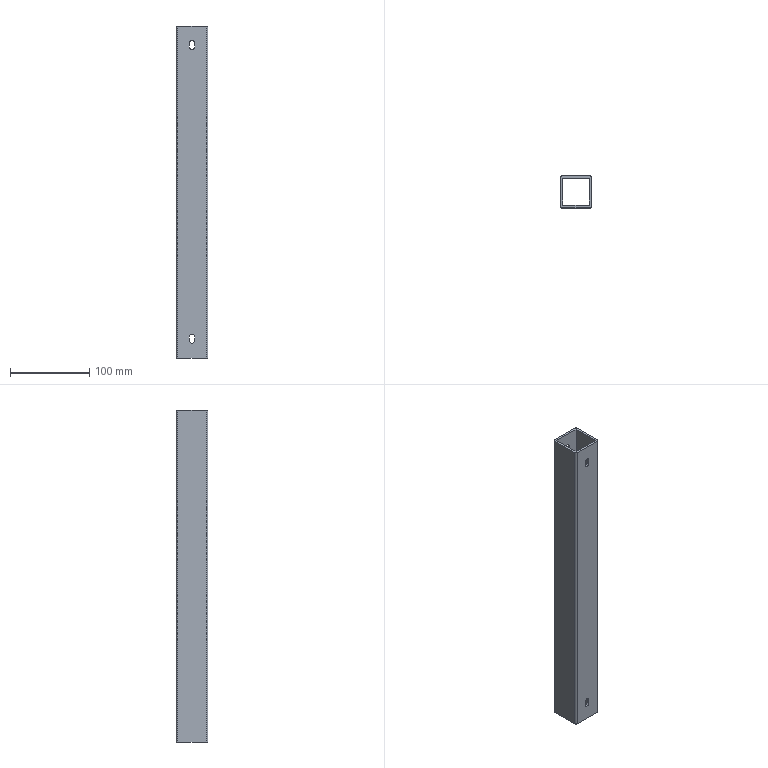Part | STEP file | X77-09102 | 1 solid | 34 faces | box 40 x 40 x 420 mm | volume 183605 mm3 | plane 18 | cylinder 16 | commonest cylinder face diameters 6.5 x6 12 x6 4 x4
STEP:
#1=CARTESIAN_POINT('',(20.,0.,401.386));
#2=VERTEX_POINT('',#1);
#3=CARTESIAN_POINT('',(23.25,0.,398.136));
#4=VERTEX_POINT('',#3);
#5=CARTESIAN_POINT('',(20.,0.,398.136));
#6=DIRECTION('',(0.,1.,0.));
#7=DIRECTION('',(0.,0.,1.));
#8=AXIS2_PLACEMENT_3D('',#5,#6,#7);
#9=CIRCLE('',#8,3.25);
#10=EDGE_CURVE('',#2,#4,#9,.T.);
#11=ORIENTED_EDGE('',*,*,#10,.F.);
#12=CARTESIAN_POINT('',(20.,3.,401.386));
#13=VERTEX_POINT('',#12);
#14=CARTESIAN_POINT('',(20.,-7.,401.386));
#15=DIRECTION('',(0.,1.,0.));
#16=VECTOR('',#15,1000.);
#17=LINE('',#14,#16);
#18=EDGE_CURVE('',#2,#13,#17,.T.);
#19=ORIENTED_EDGE('',*,*,#18,.T.);
#20=CARTESIAN_POINT('',(23.25,3.,398.136));
#21=VERTEX_POINT('',#20);
#22=CARTESIAN_POINT('',(20.,3.,398.136));
#23=DIRECTION('',(0.,1.,0.));
#24=DIRECTION('',(0.,0.,1.));
#25=AXIS2_PLACEMENT_3D('',#22,#23,#24);
#26=CIRCLE('',#25,3.25);
#27=EDGE_CURVE('',#13,#21,#26,.T.);
#28=ORIENTED_EDGE('',*,*,#27,.T.);
#29=CARTESIAN_POINT('',(23.25,-7.,398.136));
#30=DIRECTION('',(0.,1.,0.));
#31=VECTOR('',#30,1000.);
#32=LINE('',#29,#31);
#33=EDGE_CURVE('',#4,#21,#32,.T.);
#34=ORIENTED_EDGE('',*,*,#33,.F.);
#35=EDGE_LOOP('',(#11,#19,#28,#34));
#36=FACE_OUTER_BOUND('',#35,.T.);
#37=CARTESIAN_POINT('',(20.,-7.,398.136));
#38=DIRECTION('',(0.,1.,0.));
#39=DIRECTION('',(0.,0.,1.));
#40=AXIS2_PLACEMENT_3D('',#37,#38,#39);
#41=CYLINDRICAL_SURFACE('',#40,3.25);
#42=ADVANCED_FACE('',(#36),#41,.F.);
#43=CARTESIAN_POINT('',(20.,0.,30.1));
#44=VERTEX_POINT('',#43);
#45=CARTESIAN_POINT('',(23.25,0.,26.85));
#46=VERTEX_POINT('',#45);
#47=CARTESIAN_POINT('',(20.,0.,26.85));
#48=DIRECTION('',(0.,1.,0.));
#49=DIRECTION('',(0.,0.,1.));
#50=AXIS2_PLACEMENT_3D('',#47,#48,#49);
#51=CIRCLE('',#50,3.25);
#52=EDGE_CURVE('',#44,#46,#51,.T.);
#53=ORIENTED_EDGE('',*,*,#52,.F.);
#54=CARTESIAN_POINT('',(20.,3.,30.1));
#55=VERTEX_POINT('',#54);
#56=CARTESIAN_POINT('',(20.,-7.,30.1));
#57=DIRECTION('',(0.,1.,0.));
#58=VECTOR('',#57,1000.);
#59=LINE('',#56,#58);
#60=EDGE_CURVE('',#44,#55,#59,.T.);
#61=ORIENTED_EDGE('',*,*,#60,.T.);
#62=CARTESIAN_POINT('',(23.25,3.,26.85));
#63=VERTEX_POINT('',#62);
#64=CARTESIAN_POINT('',(20.,3.,26.85));
#65=DIRECTION('',(0.,1.,0.));
#66=DIRECTION('',(0.,0.,1.));
#67=AXIS2_PLACEMENT_3D('',#64,#65,#66);
#68=CIRCLE('',#67,3.25);
#69=EDGE_CURVE('',#55,#63,#68,.T.);
#70=ORIENTED_EDGE('',*,*,#69,.T.);
#71=CARTESIAN_POINT('',(23.25,-7.,26.85));
#72=DIRECTION('',(0.,1.,0.));
#73=VECTOR('',#72,1000.);
#74=LINE('',#71,#73);
#75=EDGE_CURVE('',#46,#63,#74,.T.);
#76=ORIENTED_EDGE('',*,*,#75,.F.);
#77=EDGE_LOOP('',(#53,#61,#70,#76));
#78=FACE_OUTER_BOUND('',#77,.T.);
#79=CARTESIAN_POINT('',(20.,-7.,26.85));
#80=DIRECTION('',(0.,1.,0.));
#81=DIRECTION('',(0.,0.,1.));
#82=AXIS2_PLACEMENT_3D('',#79,#80,#81);
#83=CYLINDRICAL_SURFACE('',#82,3.25);
#84=ADVANCED_FACE('',(#78),#83,.F.);
#85=CARTESIAN_POINT('',(26.,37.,398.136));
#86=VERTEX_POINT('',#85);
#87=CARTESIAN_POINT('',(20.,37.,404.136));
#88=VERTEX_POINT('',#87);
#89=CARTESIAN_POINT('',(20.,37.,398.136));
#90=DIRECTION('',(0.,-1.,0.));
#91=DIRECTION('',(0.,0.,-1.));
#92=AXIS2_PLACEMENT_3D('',#89,#90,#91);
#93=CIRCLE('',#92,6.);
#94=EDGE_CURVE('',#86,#88,#93,.T.);
#95=ORIENTED_EDGE('',*,*,#94,.T.);
#96=CARTESIAN_POINT('',(20.,40.,404.136));
#97=VERTEX_POINT('',#96);
#98=CARTESIAN_POINT('',(20.,30.,404.136));
#99=DIRECTION('',(0.,1.,0.));
#100=VECTOR('',#99,1000.);
#101=LINE('',#98,#100);
#102=EDGE_CURVE('',#88,#97,#101,.T.);
#103=ORIENTED_EDGE('',*,*,#102,.T.);
#104=CARTESIAN_POINT('',(26.,40.,398.136));
#105=VERTEX_POINT('',#104);
#106=CARTESIAN_POINT('',(20.,40.,398.136));
#107=DIRECTION('',(0.,1.,0.));
#108=DIRECTION('',(0.,0.,1.));
#109=AXIS2_PLACEMENT_3D('',#106,#107,#108);
#110=CIRCLE('',#109,6.);
#111=EDGE_CURVE('',#97,#105,#110,.T.);
#112=ORIENTED_EDGE('',*,*,#111,.T.);
#113=CARTESIAN_POINT('',(26.,30.,398.136));
#114=DIRECTION('',(0.,1.,0.));
#115=VECTOR('',#114,1000.);
#116=LINE('',#113,#115);
#117=EDGE_CURVE('',#86,#105,#116,.T.);
#118=ORIENTED_EDGE('',*,*,#117,.F.);
#119=EDGE_LOOP('',(#95,#103,#112,#118));
#120=FACE_OUTER_BOUND('',#119,.T.);
#121=CARTESIAN_POINT('',(20.,30.,398.136));
#122=DIRECTION('',(0.,1.,0.));
#123=DIRECTION('',(0.,0.,1.));
#124=AXIS2_PLACEMENT_3D('',#121,#122,#123);
#125=CYLINDRICAL_SURFACE('',#124,6.);
#126=ADVANCED_FACE('',(#120),#125,.F.);
#127=CARTESIAN_POINT('',(26.,37.,26.85));
#128=VERTEX_POINT('',#127);
#129=CARTESIAN_POINT('',(20.,37.,32.85));
#130=VERTEX_POINT('',#129);
#131=CARTESIAN_POINT('',(20.,37.,26.85));
#132=DIRECTION('',(0.,-1.,0.));
#133=DIRECTION('',(0.,0.,-1.));
#134=AXIS2_PLACEMENT_3D('',#131,#132,#133);
#135=CIRCLE('',#134,6.);
#136=EDGE_CURVE('',#128,#130,#135,.T.);
#137=ORIENTED_EDGE('',*,*,#136,.T.);
#138=CARTESIAN_POINT('',(20.,40.,32.85));
#139=VERTEX_POINT('',#138);
#140=CARTESIAN_POINT('',(20.,30.,32.85));
#141=DIRECTION('',(0.,1.,0.));
#142=VECTOR('',#141,1000.);
#143=LINE('',#140,#142);
#144=EDGE_CURVE('',#130,#139,#143,.T.);
#145=ORIENTED_EDGE('',*,*,#144,.T.);
#146=CARTESIAN_POINT('',(26.,40.,26.85));
#147=VERTEX_POINT('',#146);
#148=CARTESIAN_POINT('',(20.,40.,26.85));
#149=DIRECTION('',(0.,1.,0.));
#150=DIRECTION('',(0.,0.,1.));
#151=AXIS2_PLACEMENT_3D('',#148,#149,#150);
#152=CIRCLE('',#151,6.);
#153=EDGE_CURVE('',#139,#147,#152,.T.);
#154=ORIENTED_EDGE('',*,*,#153,.T.);
#155=CARTESIAN_POINT('',(26.,30.,26.85));
#156=DIRECTION('',(0.,1.,0.));
#157=VECTOR('',#156,1000.);
#158=LINE('',#155,#157);
#159=EDGE_CURVE('',#128,#147,#158,.T.);
#160=ORIENTED_EDGE('',*,*,#159,.F.);
#161=EDGE_LOOP('',(#137,#145,#154,#160));
#162=FACE_OUTER_BOUND('',#161,.T.);
#163=CARTESIAN_POINT('',(20.,30.,26.85));
#164=DIRECTION('',(0.,1.,0.));
#165=DIRECTION('',(0.,0.,1.));
#166=AXIS2_PLACEMENT_3D('',#163,#164,#165);
#167=CYLINDRICAL_SURFACE('',#166,6.);
#168=ADVANCED_FACE('',(#162),#167,.F.);
#169=CARTESIAN_POINT('',(0.,2.,420.));
#170=VERTEX_POINT('',#169);
#171=CARTESIAN_POINT('',(2.,0.,420.));
#172=VERTEX_POINT('',#171);
#173=CARTESIAN_POINT('',(2.,2.,420.));
#174=DIRECTION('',(0.,0.,1.));
#175=DIRECTION('',(1.,0.,0.));
#176=AXIS2_PLACEMENT_3D('',#173,#174,#175);
#177=CIRCLE('',#176,2.);
#178=EDGE_CURVE('',#170,#172,#177,.T.);
#179=ORIENTED_EDGE('',*,*,#178,.T.);
#180=CARTESIAN_POINT('',(38.,0.,420.));
#181=VERTEX_POINT('',#180);
#182=CARTESIAN_POINT('',(2.,0.,420.));
#183=DIRECTION('',(1.,0.,0.));
#184=VECTOR('',#183,1000.);
#185=LINE('',#182,#184);
#186=EDGE_CURVE('',#172,#181,#185,.T.);
#187=ORIENTED_EDGE('',*,*,#186,.T.);
#188=CARTESIAN_POINT('',(40.,2.,420.));
#189=VERTEX_POINT('',#188);
#190=CARTESIAN_POINT('',(38.,2.,420.));
#191=DIRECTION('',(0.,0.,1.));
#192=DIRECTION('',(1.,0.,0.));
#193=AXIS2_PLACEMENT_3D('',#190,#191,#192);
#194=CIRCLE('',#193,2.);
#195=EDGE_CURVE('',#181,#189,#194,.T.);
#196=ORIENTED_EDGE('',*,*,#195,.T.);
#197=CARTESIAN_POINT('',(40.,38.,420.));
#198=VERTEX_POINT('',#197);
#199=CARTESIAN_POINT('',(40.,2.,420.));
#200=DIRECTION('',(0.,1.,0.));
#201=VECTOR('',#200,1000.);
#202=LINE('',#199,#201);
#203=EDGE_CURVE('',#189,#198,#202,.T.);
#204=ORIENTED_EDGE('',*,*,#203,.T.);
#205=CARTESIAN_POINT('',(38.,40.,420.));
#206=VERTEX_POINT('',#205);
#207=CARTESIAN_POINT('',(38.,38.,420.));
#208=DIRECTION('',(0.,0.,1.));
#209=DIRECTION('',(1.,0.,0.));
#210=AXIS2_PLACEMENT_3D('',#207,#208,#209);
#211=CIRCLE('',#210,2.);
#212=EDGE_CURVE('',#198,#206,#211,.T.);
#213=ORIENTED_EDGE('',*,*,#212,.T.);
#214=CARTESIAN_POINT('',(2.,40.,420.));
#215=VERTEX_POINT('',#214);
#216=CARTESIAN_POINT('',(2.,40.,420.));
#217=DIRECTION('',(-1.,0.,0.));
#218=VECTOR('',#217,1000.);
#219=LINE('',#216,#218);
#220=EDGE_CURVE('',#206,#215,#219,.T.);
#221=ORIENTED_EDGE('',*,*,#220,.T.);
#222=CARTESIAN_POINT('',(0.,38.,420.));
#223=VERTEX_POINT('',#222);
#224=CARTESIAN_POINT('',(2.,38.,420.));
#225=DIRECTION('',(0.,0.,1.));
#226=DIRECTION('',(-1.,0.,0.));
#227=AXIS2_PLACEMENT_3D('',#224,#225,#226);
#228=CIRCLE('',#227,2.);
#229=EDGE_CURVE('',#215,#223,#228,.T.);
#230=ORIENTED_EDGE('',*,*,#229,.T.);
#231=CARTESIAN_POINT('',(0.,2.,420.));
#232=DIRECTION('',(0.,-1.,0.));
#233=VECTOR('',#232,1000.);
#234=LINE('',#231,#233);
#235=EDGE_CURVE('',#223,#170,#234,.T.);
#236=ORIENTED_EDGE('',*,*,#235,.T.);
#237=EDGE_LOOP('',(#179,#187,#196,#204,#213,#221,#230,#236));
#238=FACE_OUTER_BOUND('',#237,.T.);
#239=CARTESIAN_POINT('',(3.,3.,420.));
#240=VERTEX_POINT('',#239);
#241=CARTESIAN_POINT('',(37.,3.,420.));
#242=VERTEX_POINT('',#241);
#243=CARTESIAN_POINT('',(3.,3.,420.));
#244=DIRECTION('',(1.,0.,0.));
#245=VECTOR('',#244,1000.);
#246=LINE('',#243,#245);
#247=EDGE_CURVE('',#240,#242,#246,.T.);
#248=ORIENTED_EDGE('',*,*,#247,.F.);
#249=CARTESIAN_POINT('',(3.,37.,420.));
#250=VERTEX_POINT('',#249);
#251=CARTESIAN_POINT('',(3.,3.,420.));
#252=DIRECTION('',(0.,-1.,0.));
#253=VECTOR('',#252,1000.);
#254=LINE('',#251,#253);
#255=EDGE_CURVE('',#250,#240,#254,.T.);
#256=ORIENTED_EDGE('',*,*,#255,.F.);
#257=CARTESIAN_POINT('',(37.,37.,420.));
#258=VERTEX_POINT('',#257);
#259=CARTESIAN_POINT('',(3.,37.,420.));
#260=DIRECTION('',(-1.,0.,0.));
#261=VECTOR('',#260,1000.);
#262=LINE('',#259,#261);
#263=EDGE_CURVE('',#258,#250,#262,.T.);
#264=ORIENTED_EDGE('',*,*,#263,.F.);
#265=CARTESIAN_POINT('',(37.,3.,420.));
#266=DIRECTION('',(0.,1.,0.));
#267=VECTOR('',#266,1000.);
#268=LINE('',#265,#267);
#269=EDGE_CURVE('',#242,#258,#268,.T.);
#270=ORIENTED_EDGE('',*,*,#269,.F.);
#271=EDGE_LOOP('',(#248,#256,#264,#270));
#272=FACE_BOUND('',#271,.T.);
#273=CARTESIAN_POINT('',(2.,2.,420.));
#274=DIRECTION('',(0.,0.,1.));
#275=DIRECTION('',(1.,0.,0.));
#276=AXIS2_PLACEMENT_3D('',#273,#274,#275);
#277=PLANE('',#276);
#278=ADVANCED_FACE('',(#238,#272),#277,.T.);
#279=CARTESIAN_POINT('',(0.,2.,0.));
#280=VERTEX_POINT('',#279);
#281=CARTESIAN_POINT('',(2.,0.,0.));
#282=VERTEX_POINT('',#281);
#283=CARTESIAN_POINT('',(2.,2.,0.));
#284=DIRECTION('',(0.,0.,1.));
#285=DIRECTION('',(1.,0.,0.));
#286=AXIS2_PLACEMENT_3D('',#283,#284,#285);
#287=CIRCLE('',#286,2.);
#288=EDGE_CURVE('',#280,#282,#287,.T.);
#289=ORIENTED_EDGE('',*,*,#288,.F.);
#290=CARTESIAN_POINT('',(0.,38.,0.));
#291=VERTEX_POINT('',#290);
#292=CARTESIAN_POINT('',(0.,2.,0.));
#293=DIRECTION('',(0.,-1.,0.));
#294=VECTOR('',#293,1000.);
#295=LINE('',#292,#294);
#296=EDGE_CURVE('',#291,#280,#295,.T.);
#297=ORIENTED_EDGE('',*,*,#296,.F.);
#298=CARTESIAN_POINT('',(2.,40.,0.));
#299=VERTEX_POINT('',#298);
#300=CARTESIAN_POINT('',(2.,38.,0.));
#301=DIRECTION('',(0.,0.,1.));
#302=DIRECTION('',(-1.,0.,0.));
#303=AXIS2_PLACEMENT_3D('',#300,#301,#302);
#304=CIRCLE('',#303,2.);
#305=EDGE_CURVE('',#299,#291,#304,.T.);
#306=ORIENTED_EDGE('',*,*,#305,.F.);
#307=CARTESIAN_POINT('',(38.,40.,0.));
#308=VERTEX_POINT('',#307);
#309=CARTESIAN_POINT('',(2.,40.,0.));
#310=DIRECTION('',(-1.,0.,0.));
#311=VECTOR('',#310,1000.);
#312=LINE('',#309,#311);
#313=EDGE_CURVE('',#308,#299,#312,.T.);
#314=ORIENTED_EDGE('',*,*,#313,.F.);
#315=CARTESIAN_POINT('',(40.,38.,0.));
#316=VERTEX_POINT('',#315);
#317=CARTESIAN_POINT('',(38.,38.,0.));
#318=DIRECTION('',(0.,0.,1.));
#319=DIRECTION('',(1.,0.,0.));
#320=AXIS2_PLACEMENT_3D('',#317,#318,#319);
#321=CIRCLE('',#320,2.);
#322=EDGE_CURVE('',#316,#308,#321,.T.);
#323=ORIENTED_EDGE('',*,*,#322,.F.);
#324=CARTESIAN_POINT('',(40.,2.,0.));
#325=VERTEX_POINT('',#324);
#326=CARTESIAN_POINT('',(40.,2.,0.));
#327=DIRECTION('',(0.,1.,0.));
#328=VECTOR('',#327,1000.);
#329=LINE('',#326,#328);
#330=EDGE_CURVE('',#325,#316,#329,.T.);
#331=ORIENTED_EDGE('',*,*,#330,.F.);
#332=CARTESIAN_POINT('',(38.,0.,0.));
#333=VERTEX_POINT('',#332);
#334=CARTESIAN_POINT('',(38.,2.,0.));
#335=DIRECTION('',(0.,0.,1.));
#336=DIRECTION('',(1.,0.,0.));
#337=AXIS2_PLACEMENT_3D('',#334,#335,#336);
#338=CIRCLE('',#337,2.);
#339=EDGE_CURVE('',#333,#325,#338,.T.);
#340=ORIENTED_EDGE('',*,*,#339,.F.);
#341=CARTESIAN_POINT('',(2.,0.,0.));
#342=DIRECTION('',(1.,0.,0.));
#343=VECTOR('',#342,1000.);
#344=LINE('',#341,#343);
#345=EDGE_CURVE('',#282,#333,#344,.T.);
#346=ORIENTED_EDGE('',*,*,#345,.F.);
#347=EDGE_LOOP('',(#289,#297,#306,#314,#323,#331,#340,#346));
#348=FACE_OUTER_BOUND('',#347,.T.);
#349=CARTESIAN_POINT('',(3.,37.,0.));
#350=VERTEX_POINT('',#349);
#351=CARTESIAN_POINT('',(3.,3.,0.));
#352=VERTEX_POINT('',#351);
#353=CARTESIAN_POINT('',(3.,3.,0.));
#354=DIRECTION('',(0.,-1.,0.));
#355=VECTOR('',#354,1000.);
#356=LINE('',#353,#355);
#357=EDGE_CURVE('',#350,#352,#356,.T.);
#358=ORIENTED_EDGE('',*,*,#357,.T.);
#359=CARTESIAN_POINT('',(37.,3.,0.));
#360=VERTEX_POINT('',#359);
#361=CARTESIAN_POINT('',(3.,3.,0.));
#362=DIRECTION('',(1.,0.,0.));
#363=VECTOR('',#362,1000.);
#364=LINE('',#361,#363);
#365=EDGE_CURVE('',#352,#360,#364,.T.);
#366=ORIENTED_EDGE('',*,*,#365,.T.);
#367=CARTESIAN_POINT('',(37.,37.,0.));
#368=VERTEX_POINT('',#367);
#369=CARTESIAN_POINT('',(37.,3.,0.));
#370=DIRECTION('',(0.,1.,0.));
#371=VECTOR('',#370,1000.);
#372=LINE('',#369,#371);
#373=EDGE_CURVE('',#360,#368,#372,.T.);
#374=ORIENTED_EDGE('',*,*,#373,.T.);
#375=CARTESIAN_POINT('',(3.,37.,0.));
#376=DIRECTION('',(-1.,0.,0.));
#377=VECTOR('',#376,1000.);
#378=LINE('',#375,#377);
#379=EDGE_CURVE('',#368,#350,#378,.T.);
#380=ORIENTED_EDGE('',*,*,#379,.T.);
#381=EDGE_LOOP('',(#358,#366,#374,#380));
#382=FACE_BOUND('',#381,.T.);
#383=CARTESIAN_POINT('',(2.,2.,0.));
#384=DIRECTION('',(0.,0.,1.));
#385=DIRECTION('',(1.,0.,0.));
#386=AXIS2_PLACEMENT_3D('',#383,#384,#385);
#387=PLANE('',#386);
#388=ADVANCED_FACE('',(#348,#382),#387,.F.);
#389=ORIENTED_EDGE('',*,*,#288,.T.);
#390=CARTESIAN_POINT('',(2.,0.,420.));
#391=DIRECTION('',(0.,0.,-1.));
#392=VECTOR('',#391,1000.);
#393=LINE('',#390,#392);
#394=EDGE_CURVE('',#172,#282,#393,.T.);
#395=ORIENTED_EDGE('',*,*,#394,.F.);
#396=ORIENTED_EDGE('',*,*,#178,.F.);
#397=CARTESIAN_POINT('',(0.,2.,420.));
#398=DIRECTION('',(0.,0.,-1.));
#399=VECTOR('',#398,1000.);
#400=LINE('',#397,#399);
#401=EDGE_CURVE('',#170,#280,#400,.T.);
#402=ORIENTED_EDGE('',*,*,#401,.T.);
#403=EDGE_LOOP('',(#389,#395,#396,#402));
#404=FACE_OUTER_BOUND('',#403,.T.);
#405=CARTESIAN_POINT('',(2.,2.,420.));
#406=DIRECTION('',(0.,0.,-1.));
#407=DIRECTION('',(-1.,0.,0.));
#408=AXIS2_PLACEMENT_3D('',#405,#406,#407);
#409=CYLINDRICAL_SURFACE('',#408,2.);
#410=ADVANCED_FACE('',(#404),#409,.T.);
#411=CARTESIAN_POINT('',(16.75,0.,393.136));
#412=VERTEX_POINT('',#411);
#413=CARTESIAN_POINT('',(16.75,0.,398.136));
#414=VERTEX_POINT('',#413);
#415=CARTESIAN_POINT('',(16.75,0.,420.));
#416=DIRECTION('',(0.,0.,1.));
#417=VECTOR('',#416,1000.);
#418=LINE('',#415,#417);
#419=EDGE_CURVE('',#412,#414,#418,.T.);
#420=ORIENTED_EDGE('',*,*,#419,.T.);
#421=CARTESIAN_POINT('',(20.,0.,398.136));
#422=DIRECTION('',(0.,1.,0.));
#423=DIRECTION('',(0.,0.,1.));
#424=AXIS2_PLACEMENT_3D('',#421,#422,#423);
#425=CIRCLE('',#424,3.25);
#426=EDGE_CURVE('',#414,#2,#425,.T.);
#427=ORIENTED_EDGE('',*,*,#426,.T.);
#428=ORIENTED_EDGE('',*,*,#10,.T.);
#429=CARTESIAN_POINT('',(23.25,0.,393.136));
#430=VERTEX_POINT('',#429);
#431=CARTESIAN_POINT('',(23.25,0.,420.));
#432=DIRECTION('',(0.,0.,-1.));
#433=VECTOR('',#432,1000.);
#434=LINE('',#431,#433);
#435=EDGE_CURVE('',#4,#430,#434,.T.);
#436=ORIENTED_EDGE('',*,*,#435,.T.);
#437=CARTESIAN_POINT('',(20.,0.,393.136));
#438=DIRECTION('',(0.,1.,0.));
#439=DIRECTION('',(0.,0.,1.));
#440=AXIS2_PLACEMENT_3D('',#437,#438,#439);
#441=CIRCLE('',#440,3.25);
#442=EDGE_CURVE('',#430,#412,#441,.T.);
#443=ORIENTED_EDGE('',*,*,#442,.T.);
#444=EDGE_LOOP('',(#420,#427,#428,#436,#443));
#445=FACE_BOUND('',#444,.T.);
#446=CARTESIAN_POINT('',(23.25,0.,21.85));
#447=VERTEX_POINT('',#446);
#448=CARTESIAN_POINT('',(23.25,0.,420.));
#449=DIRECTION('',(0.,0.,-1.));
#450=VECTOR('',#449,1000.);
#451=LINE('',#448,#450);
#452=EDGE_CURVE('',#46,#447,#451,.T.);
#453=ORIENTED_EDGE('',*,*,#452,.T.);
#454=CARTESIAN_POINT('',(16.75,0.,21.85));
#455=VERTEX_POINT('',#454);
#456=CARTESIAN_POINT('',(20.,0.,21.85));
#457=DIRECTION('',(0.,1.,0.));
#458=DIRECTION('',(0.,0.,1.));
#459=AXIS2_PLACEMENT_3D('',#456,#457,#458);
#460=CIRCLE('',#459,3.25);
#461=EDGE_CURVE('',#447,#455,#460,.T.);
#462=ORIENTED_EDGE('',*,*,#461,.T.);
#463=CARTESIAN_POINT('',(16.75,0.,26.85));
#464=VERTEX_POINT('',#463);
#465=CARTESIAN_POINT('',(16.75,0.,420.));
#466=DIRECTION('',(0.,0.,1.));
#467=VECTOR('',#466,1000.);
#468=LINE('',#465,#467);
#469=EDGE_CURVE('',#455,#464,#468,.T.);
#470=ORIENTED_EDGE('',*,*,#469,.T.);
#471=CARTESIAN_POINT('',(20.,0.,26.85));
#472=DIRECTION('',(0.,1.,0.));
#473=DIRECTION('',(0.,0.,1.));
#474=AXIS2_PLACEMENT_3D('',#471,#472,#473);
#475=CIRCLE('',#474,3.25);
#476=EDGE_CURVE('',#464,#44,#475,.T.);
#477=ORIENTED_EDGE('',*,*,#476,.T.);
#478=ORIENTED_EDGE('',*,*,#52,.T.);
#479=EDGE_LOOP('',(#453,#462,#470,#477,#478));
#480=FACE_BOUND('',#479,.T.);
#481=ORIENTED_EDGE('',*,*,#345,.T.);
#482=CARTESIAN_POINT('',(38.,0.,420.));
#483=DIRECTION('',(0.,0.,-1.));
#484=VECTOR('',#483,1000.);
#485=LINE('',#482,#484);
#486=EDGE_CURVE('',#181,#333,#485,.T.);
#487=ORIENTED_EDGE('',*,*,#486,.F.);
#488=ORIENTED_EDGE('',*,*,#186,.F.);
#489=ORIENTED_EDGE('',*,*,#394,.T.);
#490=EDGE_LOOP('',(#481,#487,#488,#489));
#491=FACE_OUTER_BOUND('',#490,.T.);
#492=CARTESIAN_POINT('',(2.,0.,420.));
#493=DIRECTION('',(0.,1.,0.));
#494=DIRECTION('',(0.,0.,1.));
#495=AXIS2_PLACEMENT_3D('',#492,#493,#494);
#496=PLANE('',#495);
#497=ADVANCED_FACE('',(#445,#480,#491),#496,.F.);
#498=ORIENTED_EDGE('',*,*,#339,.T.);
#499=CARTESIAN_POINT('',(40.,2.,420.));
#500=DIRECTION('',(0.,0.,-1.));
#501=VECTOR('',#500,1000.);
#502=LINE('',#499,#501);
#503=EDGE_CURVE('',#189,#325,#502,.T.);
#504=ORIENTED_EDGE('',*,*,#503,.F.);
#505=ORIENTED_EDGE('',*,*,#195,.F.);
#506=ORIENTED_EDGE('',*,*,#486,.T.);
#507=EDGE_LOOP('',(#498,#504,#505,#506));
#508=FACE_OUTER_BOUND('',#507,.T.);
#509=CARTESIAN_POINT('',(38.,2.,420.));
#510=DIRECTION('',(0.,0.,-1.));
#511=DIRECTION('',(-1.,0.,0.));
#512=AXIS2_PLACEMENT_3D('',#509,#510,#511);
#513=CYLINDRICAL_SURFACE('',#512,2.);
#514=ADVANCED_FACE('',(#508),#513,.T.);
#515=ORIENTED_EDGE('',*,*,#330,.T.);
#516=CARTESIAN_POINT('',(40.,38.,420.));
#517=DIRECTION('',(0.,0.,-1.));
#518=VECTOR('',#517,1000.);
#519=LINE('',#516,#518);
#520=EDGE_CURVE('',#198,#316,#519,.T.);
#521=ORIENTED_EDGE('',*,*,#520,.F.);
#522=ORIENTED_EDGE('',*,*,#203,.F.);
#523=ORIENTED_EDGE('',*,*,#503,.T.);
#524=EDGE_LOOP('',(#515,#521,#522,#523));
#525=FACE_OUTER_BOUND('',#524,.T.);
#526=CARTESIAN_POINT('',(40.,2.,420.));
#527=DIRECTION('',(-1.,0.,0.));
#528=DIRECTION('',(0.,-1.,0.));
#529=AXIS2_PLACEMENT_3D('',#526,#527,#528);
#530=PLANE('',#529);
#531=ADVANCED_FACE('',(#525),#530,.F.);
#532=ORIENTED_EDGE('',*,*,#322,.T.);
#533=CARTESIAN_POINT('',(38.,40.,420.));
#534=DIRECTION('',(0.,0.,-1.));
#535=VECTOR('',#534,1000.);
#536=LINE('',#533,#535);
#537=EDGE_CURVE('',#206,#308,#536,.T.);
#538=ORIENTED_EDGE('',*,*,#537,.F.);
#539=ORIENTED_EDGE('',*,*,#212,.F.);
#540=ORIENTED_EDGE('',*,*,#520,.T.);
#541=EDGE_LOOP('',(#532,#538,#539,#540));
#542=FACE_OUTER_BOUND('',#541,.T.);
#543=CARTESIAN_POINT('',(38.,38.,420.));
#544=DIRECTION('',(0.,0.,-1.));
#545=DIRECTION('',(-1.,0.,0.));
#546=AXIS2_PLACEMENT_3D('',#543,#544,#545);
#547=CYLINDRICAL_SURFACE('',#546,2.);
#548=ADVANCED_FACE('',(#542),#547,.T.);
#549=CARTESIAN_POINT('',(14.,40.,393.136));
#550=VERTEX_POINT('',#549);
#551=CARTESIAN_POINT('',(14.,40.,398.136));
#552=VERTEX_POINT('',#551);
#553=CARTESIAN_POINT('',(14.,40.,393.136));
#554=DIRECTION('',(0.,0.,1.));
#555=VECTOR('',#554,1000.);
#556=LINE('',#553,#555);
#557=EDGE_CURVE('',#550,#552,#556,.T.);
#558=ORIENTED_EDGE('',*,*,#557,.F.);
#559=CARTESIAN_POINT('',(26.,40.,393.136));
#560=VERTEX_POINT('',#559);
#561=CARTESIAN_POINT('',(20.,40.,393.136));
#562=DIRECTION('',(0.,1.,0.));
#563=DIRECTION('',(0.,0.,1.));
#564=AXIS2_PLACEMENT_3D('',#561,#562,#563);
#565=CIRCLE('',#564,6.);
#566=EDGE_CURVE('',#560,#550,#565,.T.);
#567=ORIENTED_EDGE('',*,*,#566,.F.);
#568=CARTESIAN_POINT('',(26.,40.,393.136));
#569=DIRECTION('',(0.,0.,-1.));
#570=VECTOR('',#569,1000.);
#571=LINE('',#568,#570);
#572=EDGE_CURVE('',#105,#560,#571,.T.);
#573=ORIENTED_EDGE('',*,*,#572,.F.);
#574=ORIENTED_EDGE('',*,*,#111,.F.);
#575=CARTESIAN_POINT('',(20.,40.,398.136));
#576=DIRECTION('',(0.,1.,0.));
#577=DIRECTION('',(0.,0.,1.));
#578=AXIS2_PLACEMENT_3D('',#575,#576,#577);
#579=CIRCLE('',#578,6.);
#580=EDGE_CURVE('',#552,#97,#579,.T.);
#581=ORIENTED_EDGE('',*,*,#580,.F.);
#582=EDGE_LOOP('',(#558,#567,#573,#574,#581));
#583=FACE_BOUND('',#582,.T.);
#584=CARTESIAN_POINT('',(14.,40.,21.85));
#585=VERTEX_POINT('',#584);
#586=CARTESIAN_POINT('',(14.,40.,26.85));
#587=VERTEX_POINT('',#586);
#588=CARTESIAN_POINT('',(14.,40.,21.85));
#589=DIRECTION('',(0.,0.,1.));
#590=VECTOR('',#589,1000.);
#591=LINE('',#588,#590);
#592=EDGE_CURVE('',#585,#587,#591,.T.);
#593=ORIENTED_EDGE('',*,*,#592,.F.);
#594=CARTESIAN_POINT('',(26.,40.,21.85));
#595=VERTEX_POINT('',#594);
#596=CARTESIAN_POINT('',(20.,40.,21.85));
#597=DIRECTION('',(0.,1.,0.));
#598=DIRECTION('',(0.,0.,1.));
#599=AXIS2_PLACEMENT_3D('',#596,#597,#598);
#600=CIRCLE('',#599,6.);
#601=EDGE_CURVE('',#595,#585,#600,.T.);
#602=ORIENTED_EDGE('',*,*,#601,.F.);
#603=CARTESIAN_POINT('',(26.,40.,21.85));
#604=DIRECTION('',(0.,0.,-1.));
#605=VECTOR('',#604,1000.);
#606=LINE('',#603,#605);
#607=EDGE_CURVE('',#147,#595,#606,.T.);
#608=ORIENTED_EDGE('',*,*,#607,.F.);
#609=ORIENTED_EDGE('',*,*,#153,.F.);
#610=CARTESIAN_POINT('',(20.,40.,26.85));
#611=DIRECTION('',(0.,1.,0.));
#612=DIRECTION('',(0.,0.,1.));
#613=AXIS2_PLACEMENT_3D('',#610,#611,#612);
#614=CIRCLE('',#613,6.);
#615=EDGE_CURVE('',#587,#139,#614,.T.);
#616=ORIENTED_EDGE('',*,*,#615,.F.);
#617=EDGE_LOOP('',(#593,#602,#608,#609,#616));
#618=FACE_BOUND('',#617,.T.);
#619=ORIENTED_EDGE('',*,*,#313,.T.);
#620=CARTESIAN_POINT('',(2.,40.,420.));
#621=DIRECTION('',(0.,0.,-1.));
#622=VECTOR('',#621,1000.);
#623=LINE('',#620,#622);
#624=EDGE_CURVE('',#215,#299,#623,.T.);
#625=ORIENTED_EDGE('',*,*,#624,.F.);
#626=ORIENTED_EDGE('',*,*,#220,.F.);
#627=ORIENTED_EDGE('',*,*,#537,.T.);
#628=EDGE_LOOP('',(#619,#625,#626,#627));
#629=FACE_OUTER_BOUND('',#628,.T.);
#630=CARTESIAN_POINT('',(2.,40.,420.));
#631=DIRECTION('',(0.,-1.,0.));
#632=DIRECTION('',(0.,0.,-1.));
#633=AXIS2_PLACEMENT_3D('',#630,#631,#632);
#634=PLANE('',#633);
#635=ADVANCED_FACE('',(#583,#618,#629),#634,.F.);
#636=ORIENTED_EDGE('',*,*,#305,.T.);
#637=CARTESIAN_POINT('',(0.,38.,420.));
#638=DIRECTION('',(0.,0.,-1.));
#639=VECTOR('',#638,1000.);
#640=LINE('',#637,#639);
#641=EDGE_CURVE('',#223,#291,#640,.T.);
#642=ORIENTED_EDGE('',*,*,#641,.F.);
#643=ORIENTED_EDGE('',*,*,#229,.F.);
#644=ORIENTED_EDGE('',*,*,#624,.T.);
#645=EDGE_LOOP('',(#636,#642,#643,#644));
#646=FACE_OUTER_BOUND('',#645,.T.);
#647=CARTESIAN_POINT('',(2.,38.,420.));
#648=DIRECTION('',(0.,0.,-1.));
#649=DIRECTION('',(-1.,0.,0.));
#650=AXIS2_PLACEMENT_3D('',#647,#648,#649);
#651=CYLINDRICAL_SURFACE('',#650,2.);
#652=ADVANCED_FACE('',(#646),#651,.T.);
#653=ORIENTED_EDGE('',*,*,#296,.T.);
#654=ORIENTED_EDGE('',*,*,#401,.F.);
#655=ORIENTED_EDGE('',*,*,#235,.F.);
#656=ORIENTED_EDGE('',*,*,#641,.T.);
#657=EDGE_LOOP('',(#653,#654,#655,#656));
#658=FACE_OUTER_BOUND('',#657,.T.);
#659=CARTESIAN_POINT('',(0.,2.,420.));
#660=DIRECTION('',(1.,0.,0.));
#661=DIRECTION('',(0.,1.,0.));
#662=AXIS2_PLACEMENT_3D('',#659,#660,#661);
#663=PLANE('',#662);
#664=ADVANCED_FACE('',(#658),#663,.F.);
#665=ORIENTED_EDGE('',*,*,#357,.F.);
#666=CARTESIAN_POINT('',(3.,37.,420.));
#667=DIRECTION('',(0.,0.,-1.));
#668=VECTOR('',#667,1000.);
#669=LINE('',#666,#668);
#670=EDGE_CURVE('',#250,#350,#669,.T.);
#671=ORIENTED_EDGE('',*,*,#670,.F.);
#672=ORIENTED_EDGE('',*,*,#255,.T.);
#673=CARTESIAN_POINT('',(3.,3.,420.));
#674=DIRECTION('',(0.,0.,-1.));
#675=VECTOR('',#674,1000.);
#676=LINE('',#673,#675);
#677=EDGE_CURVE('',#240,#352,#676,.T.);
#678=ORIENTED_EDGE('',*,*,#677,.T.);
#679=EDGE_LOOP('',(#665,#671,#672,#678));
#680=FACE_OUTER_BOUND('',#679,.T.);
#681=CARTESIAN_POINT('',(3.,3.,420.));
#682=DIRECTION('',(1.,0.,0.));
#683=DIRECTION('',(0.,0.,-1.));
#684=AXIS2_PLACEMENT_3D('',#681,#682,#683);
#685=PLANE('',#684);
#686=ADVANCED_FACE('',(#680),#685,.T.);
#687=CARTESIAN_POINT('',(16.75,3.,398.136));
#688=VERTEX_POINT('',#687);
#689=CARTESIAN_POINT('',(20.,3.,398.136));
#690=DIRECTION('',(0.,1.,0.));
#691=DIRECTION('',(0.,0.,1.));
#692=AXIS2_PLACEMENT_3D('',#689,#690,#691);
#693=CIRCLE('',#692,3.25);
#694=EDGE_CURVE('',#688,#13,#693,.T.);
#695=ORIENTED_EDGE('',*,*,#694,.F.);
#696=CARTESIAN_POINT('',(16.75,3.,393.136));
#697=VERTEX_POINT('',#696);
#698=CARTESIAN_POINT('',(16.75,3.,398.136));
#699=DIRECTION('',(0.,0.,1.));
#700=VECTOR('',#699,1000.);
#701=LINE('',#698,#700);
#702=EDGE_CURVE('',#697,#688,#701,.T.);
#703=ORIENTED_EDGE('',*,*,#702,.F.);
#704=CARTESIAN_POINT('',(23.25,3.,393.136));
#705=VERTEX_POINT('',#704);
#706=CARTESIAN_POINT('',(20.,3.,393.136));
#707=DIRECTION('',(0.,1.,0.));
#708=DIRECTION('',(0.,0.,1.));
#709=AXIS2_PLACEMENT_3D('',#706,#707,#708);
#710=CIRCLE('',#709,3.25);
#711=EDGE_CURVE('',#705,#697,#710,.T.);
#712=ORIENTED_EDGE('',*,*,#711,.F.);
#713=CARTESIAN_POINT('',(23.25,3.,398.136));
#714=DIRECTION('',(0.,0.,-1.));
#715=VECTOR('',#714,1000.);
#716=LINE('',#713,#715);
#717=EDGE_CURVE('',#21,#705,#716,.T.);
#718=ORIENTED_EDGE('',*,*,#717,.F.);
#719=ORIENTED_EDGE('',*,*,#27,.F.);
#720=EDGE_LOOP('',(#695,#703,#712,#718,#719));
#721=FACE_BOUND('',#720,.T.);
#722=CARTESIAN_POINT('',(23.25,3.,21.85));
#723=VERTEX_POINT('',#722);
#724=CARTESIAN_POINT('',(16.75,3.,21.85));
#725=VERTEX_POINT('',#724);
#726=CARTESIAN_POINT('',(20.,3.,21.85));
#727=DIRECTION('',(0.,1.,0.));
#728=DIRECTION('',(0.,0.,1.));
#729=AXIS2_PLACEMENT_3D('',#726,#727,#728);
#730=CIRCLE('',#729,3.25);
#731=EDGE_CURVE('',#723,#725,#730,.T.);
#732=ORIENTED_EDGE('',*,*,#731,.F.);
#733=CARTESIAN_POINT('',(23.25,3.,21.85));
#734=DIRECTION('',(0.,0.,-1.));
#735=VECTOR('',#734,1000.);
#736=LINE('',#733,#735);
#737=EDGE_CURVE('',#63,#723,#736,.T.);
#738=ORIENTED_EDGE('',*,*,#737,.F.);
#739=ORIENTED_EDGE('',*,*,#69,.F.);
#740=CARTESIAN_POINT('',(16.75,3.,26.85));
#741=VERTEX_POINT('',#740);
#742=CARTESIAN_POINT('',(20.,3.,26.85));
#743=DIRECTION('',(0.,1.,0.));
#744=DIRECTION('',(0.,0.,1.));
#745=AXIS2_PLACEMENT_3D('',#742,#743,#744);
#746=CIRCLE('',#745,3.25);
#747=EDGE_CURVE('',#741,#55,#746,.T.);
#748=ORIENTED_EDGE('',*,*,#747,.F.);
#749=CARTESIAN_POINT('',(16.75,3.,21.85));
#750=DIRECTION('',(0.,0.,1.));
#751=VECTOR('',#750,1000.);
#752=LINE('',#749,#751);
#753=EDGE_CURVE('',#725,#741,#752,.T.);
#754=ORIENTED_EDGE('',*,*,#753,.F.);
#755=EDGE_LOOP('',(#732,#738,#739,#748,#754));
#756=FACE_BOUND('',#755,.T.);
#757=ORIENTED_EDGE('',*,*,#365,.F.);
#758=ORIENTED_EDGE('',*,*,#677,.F.);
#759=ORIENTED_EDGE('',*,*,#247,.T.);
#760=CARTESIAN_POINT('',(37.,3.,420.));
#761=DIRECTION('',(0.,0.,-1.));
#762=VECTOR('',#761,1000.);
#763=LINE('',#760,#762);
#764=EDGE_CURVE('',#242,#360,#763,.T.);
#765=ORIENTED_EDGE('',*,*,#764,.T.);
#766=EDGE_LOOP('',(#757,#758,#759,#765));
#767=FACE_OUTER_BOUND('',#766,.T.);
#768=CARTESIAN_POINT('',(3.,3.,420.));
#769=DIRECTION('',(0.,1.,0.));
#770=DIRECTION('',(0.,0.,1.));
#771=AXIS2_PLACEMENT_3D('',#768,#769,#770);
#772=PLANE('',#771);
#773=ADVANCED_FACE('',(#721,#756,#767),#772,.T.);
#774=ORIENTED_EDGE('',*,*,#373,.F.);
#775=ORIENTED_EDGE('',*,*,#764,.F.);
#776=ORIENTED_EDGE('',*,*,#269,.T.);
#777=CARTESIAN_POINT('',(37.,37.,420.));
#778=DIRECTION('',(0.,0.,-1.));
#779=VECTOR('',#778,1000.);
#780=LINE('',#777,#779);
#781=EDGE_CURVE('',#258,#368,#780,.T.);
#782=ORIENTED_EDGE('',*,*,#781,.T.);
#783=EDGE_LOOP('',(#774,#775,#776,#782));
#784=FACE_OUTER_BOUND('',#783,.T.);
#785=CARTESIAN_POINT('',(37.,3.,420.));
#786=DIRECTION('',(-1.,0.,0.));
#787=DIRECTION('',(0.,0.,1.));
#788=AXIS2_PLACEMENT_3D('',#785,#786,#787);
#789=PLANE('',#788);
#790=ADVANCED_FACE('',(#784),#789,.T.);
#791=CARTESIAN_POINT('',(14.,37.,393.136));
#792=VERTEX_POINT('',#791);
#793=CARTESIAN_POINT('',(26.,37.,393.136));
#794=VERTEX_POINT('',#793);
#795=CARTESIAN_POINT('',(20.,37.,393.136));
#796=DIRECTION('',(0.,-1.,0.));
#797=DIRECTION('',(0.,0.,-1.));
#798=AXIS2_PLACEMENT_3D('',#795,#796,#797);
#799=CIRCLE('',#798,6.);
#800=EDGE_CURVE('',#792,#794,#799,.T.);
#801=ORIENTED_EDGE('',*,*,#800,.F.);
#802=CARTESIAN_POINT('',(14.,37.,398.136));
#803=VERTEX_POINT('',#802);
#804=CARTESIAN_POINT('',(14.,37.,420.));
#805=DIRECTION('',(0.,0.,-1.));
#806=VECTOR('',#805,1000.);
#807=LINE('',#804,#806);
#808=EDGE_CURVE('',#803,#792,#807,.T.);
#809=ORIENTED_EDGE('',*,*,#808,.F.);
#810=CARTESIAN_POINT('',(20.,37.,398.136));
#811=DIRECTION('',(0.,-1.,0.));
#812=DIRECTION('',(0.,0.,-1.));
#813=AXIS2_PLACEMENT_3D('',#810,#811,#812);
#814=CIRCLE('',#813,6.);
#815=EDGE_CURVE('',#88,#803,#814,.T.);
#816=ORIENTED_EDGE('',*,*,#815,.F.);
#817=ORIENTED_EDGE('',*,*,#94,.F.);
#818=CARTESIAN_POINT('',(26.,37.,420.));
#819=DIRECTION('',(0.,0.,1.));
#820=VECTOR('',#819,1000.);
#821=LINE('',#818,#820);
#822=EDGE_CURVE('',#794,#86,#821,.T.);
#823=ORIENTED_EDGE('',*,*,#822,.F.);
#824=EDGE_LOOP('',(#801,#809,#816,#817,#823));
#825=FACE_BOUND('',#824,.T.);
#826=CARTESIAN_POINT('',(14.,37.,21.85));
#827=VERTEX_POINT('',#826);
#828=CARTESIAN_POINT('',(26.,37.,21.85));
#829=VERTEX_POINT('',#828);
#830=CARTESIAN_POINT('',(20.,37.,21.85));
#831=DIRECTION('',(0.,-1.,0.));
#832=DIRECTION('',(0.,0.,-1.));
#833=AXIS2_PLACEMENT_3D('',#830,#831,#832);
#834=CIRCLE('',#833,6.);
#835=EDGE_CURVE('',#827,#829,#834,.T.);
#836=ORIENTED_EDGE('',*,*,#835,.F.);
#837=CARTESIAN_POINT('',(14.,37.,26.85));
#838=VERTEX_POINT('',#837);
#839=CARTESIAN_POINT('',(14.,37.,420.));
#840=DIRECTION('',(0.,0.,-1.));
#841=VECTOR('',#840,1000.);
#842=LINE('',#839,#841);
#843=EDGE_CURVE('',#838,#827,#842,.T.);
#844=ORIENTED_EDGE('',*,*,#843,.F.);
#845=CARTESIAN_POINT('',(20.,37.,26.85));
#846=DIRECTION('',(0.,-1.,0.));
#847=DIRECTION('',(0.,0.,-1.));
#848=AXIS2_PLACEMENT_3D('',#845,#846,#847);
#849=CIRCLE('',#848,6.);
#850=EDGE_CURVE('',#130,#838,#849,.T.);
#851=ORIENTED_EDGE('',*,*,#850,.F.);
#852=ORIENTED_EDGE('',*,*,#136,.F.);
#853=CARTESIAN_POINT('',(26.,37.,420.));
#854=DIRECTION('',(0.,0.,1.));
#855=VECTOR('',#854,1000.);
#856=LINE('',#853,#855);
#857=EDGE_CURVE('',#829,#128,#856,.T.);
#858=ORIENTED_EDGE('',*,*,#857,.F.);
#859=EDGE_LOOP('',(#836,#844,#851,#852,#858));
#860=FACE_BOUND('',#859,.T.);
#861=ORIENTED_EDGE('',*,*,#379,.F.);
#862=ORIENTED_EDGE('',*,*,#781,.F.);
#863=ORIENTED_EDGE('',*,*,#263,.T.);
#864=ORIENTED_EDGE('',*,*,#670,.T.);
#865=EDGE_LOOP('',(#861,#862,#863,#864));
#866=FACE_OUTER_BOUND('',#865,.T.);
#867=CARTESIAN_POINT('',(3.,37.,420.));
#868=DIRECTION('',(0.,-1.,0.));
#869=DIRECTION('',(0.,0.,-1.));
#870=AXIS2_PLACEMENT_3D('',#867,#868,#869);
#871=PLANE('',#870);
#872=ADVANCED_FACE('',(#825,#860,#866),#871,.T.);
#873=ORIENTED_EDGE('',*,*,#835,.T.);
#874=CARTESIAN_POINT('',(26.,30.,21.85));
#875=DIRECTION('',(0.,1.,0.));
#876=VECTOR('',#875,1000.);
#877=LINE('',#874,#876);
#878=EDGE_CURVE('',#829,#595,#877,.T.);
#879=ORIENTED_EDGE('',*,*,#878,.T.);
#880=ORIENTED_EDGE('',*,*,#601,.T.);
#881=CARTESIAN_POINT('',(14.,30.,21.85));
#882=DIRECTION('',(0.,1.,0.));
#883=VECTOR('',#882,1000.);
#884=LINE('',#881,#883);
#885=EDGE_CURVE('',#827,#585,#884,.T.);
#886=ORIENTED_EDGE('',*,*,#885,.F.);
#887=EDGE_LOOP('',(#873,#879,#880,#886));
#888=FACE_OUTER_BOUND('',#887,.T.);
#889=CARTESIAN_POINT('',(20.,30.,21.85));
#890=DIRECTION('',(0.,1.,0.));
#891=DIRECTION('',(0.,0.,1.));
#892=AXIS2_PLACEMENT_3D('',#889,#890,#891);
#893=CYLINDRICAL_SURFACE('',#892,6.);
#894=ADVANCED_FACE('',(#888),#893,.F.);
#895=ORIENTED_EDGE('',*,*,#857,.T.);
#896=ORIENTED_EDGE('',*,*,#159,.T.);
#897=ORIENTED_EDGE('',*,*,#607,.T.);
#898=ORIENTED_EDGE('',*,*,#878,.F.);
#899=EDGE_LOOP('',(#895,#896,#897,#898));
#900=FACE_OUTER_BOUND('',#899,.T.);
#901=CARTESIAN_POINT('',(26.,30.,21.85));
#902=DIRECTION('',(1.,0.,0.));
#903=DIRECTION('',(0.,0.,-1.));
#904=AXIS2_PLACEMENT_3D('',#901,#902,#903);
#905=PLANE('',#904);
#906=ADVANCED_FACE('',(#900),#905,.F.);
#907=ORIENTED_EDGE('',*,*,#144,.F.);
#908=ORIENTED_EDGE('',*,*,#850,.T.);
#909=CARTESIAN_POINT('',(14.,30.,26.85));
#910=DIRECTION('',(0.,1.,0.));
#911=VECTOR('',#910,1000.);
#912=LINE('',#909,#911);
#913=EDGE_CURVE('',#838,#587,#912,.T.);
#914=ORIENTED_EDGE('',*,*,#913,.T.);
#915=ORIENTED_EDGE('',*,*,#615,.T.);
#916=EDGE_LOOP('',(#907,#908,#914,#915));
#917=FACE_OUTER_BOUND('',#916,.T.);
#918=CARTESIAN_POINT('',(20.,30.,26.85));
#919=DIRECTION('',(0.,1.,0.));
#920=DIRECTION('',(0.,0.,1.));
#921=AXIS2_PLACEMENT_3D('',#918,#919,#920);
#922=CYLINDRICAL_SURFACE('',#921,6.);
#923=ADVANCED_FACE('',(#917),#922,.F.);
#924=ORIENTED_EDGE('',*,*,#843,.T.);
#925=ORIENTED_EDGE('',*,*,#885,.T.);
#926=ORIENTED_EDGE('',*,*,#592,.T.);
#927=ORIENTED_EDGE('',*,*,#913,.F.);
#928=EDGE_LOOP('',(#924,#925,#926,#927));
#929=FACE_OUTER_BOUND('',#928,.T.);
#930=CARTESIAN_POINT('',(14.,30.,21.85));
#931=DIRECTION('',(-1.,0.,0.));
#932=DIRECTION('',(0.,0.,1.));
#933=AXIS2_PLACEMENT_3D('',#930,#931,#932);
#934=PLANE('',#933);
#935=ADVANCED_FACE('',(#929),#934,.F.);
#936=ORIENTED_EDGE('',*,*,#800,.T.);
#937=CARTESIAN_POINT('',(26.,30.,393.136));
#938=DIRECTION('',(0.,1.,0.));
#939=VECTOR('',#938,1000.);
#940=LINE('',#937,#939);
#941=EDGE_CURVE('',#794,#560,#940,.T.);
#942=ORIENTED_EDGE('',*,*,#941,.T.);
#943=ORIENTED_EDGE('',*,*,#566,.T.);
#944=CARTESIAN_POINT('',(14.,30.,393.136));
#945=DIRECTION('',(0.,1.,0.));
#946=VECTOR('',#945,1000.);
#947=LINE('',#944,#946);
#948=EDGE_CURVE('',#792,#550,#947,.T.);
#949=ORIENTED_EDGE('',*,*,#948,.F.);
#950=EDGE_LOOP('',(#936,#942,#943,#949));
#951=FACE_OUTER_BOUND('',#950,.T.);
#952=CARTESIAN_POINT('',(20.,30.,393.136));
#953=DIRECTION('',(0.,1.,0.));
#954=DIRECTION('',(0.,0.,1.));
#955=AXIS2_PLACEMENT_3D('',#952,#953,#954);
#956=CYLINDRICAL_SURFACE('',#955,6.);
#957=ADVANCED_FACE('',(#951),#956,.F.);
#958=ORIENTED_EDGE('',*,*,#822,.T.);
#959=ORIENTED_EDGE('',*,*,#117,.T.);
#960=ORIENTED_EDGE('',*,*,#572,.T.);
#961=ORIENTED_EDGE('',*,*,#941,.F.);
#962=EDGE_LOOP('',(#958,#959,#960,#961));
#963=FACE_OUTER_BOUND('',#962,.T.);
#964=CARTESIAN_POINT('',(26.,30.,393.136));
#965=DIRECTION('',(1.,0.,0.));
#966=DIRECTION('',(0.,0.,-1.));
#967=AXIS2_PLACEMENT_3D('',#964,#965,#966);
#968=PLANE('',#967);
#969=ADVANCED_FACE('',(#963),#968,.F.);
#970=ORIENTED_EDGE('',*,*,#102,.F.);
#971=ORIENTED_EDGE('',*,*,#815,.T.);
#972=CARTESIAN_POINT('',(14.,30.,398.136));
#973=DIRECTION('',(0.,1.,0.));
#974=VECTOR('',#973,1000.);
#975=LINE('',#972,#974);
#976=EDGE_CURVE('',#803,#552,#975,.T.);
#977=ORIENTED_EDGE('',*,*,#976,.T.);
#978=ORIENTED_EDGE('',*,*,#580,.T.);
#979=EDGE_LOOP('',(#970,#971,#977,#978));
#980=FACE_OUTER_BOUND('',#979,.T.);
#981=CARTESIAN_POINT('',(20.,30.,398.136));
#982=DIRECTION('',(0.,1.,0.));
#983=DIRECTION('',(0.,0.,1.));
#984=AXIS2_PLACEMENT_3D('',#981,#982,#983);
#985=CYLINDRICAL_SURFACE('',#984,6.);
#986=ADVANCED_FACE('',(#980),#985,.F.);
#987=ORIENTED_EDGE('',*,*,#808,.T.);
#988=ORIENTED_EDGE('',*,*,#948,.T.);
#989=ORIENTED_EDGE('',*,*,#557,.T.);
#990=ORIENTED_EDGE('',*,*,#976,.F.);
#991=EDGE_LOOP('',(#987,#988,#989,#990));
#992=FACE_OUTER_BOUND('',#991,.T.);
#993=CARTESIAN_POINT('',(14.,30.,393.136));
#994=DIRECTION('',(-1.,0.,0.));
#995=DIRECTION('',(0.,0.,1.));
#996=AXIS2_PLACEMENT_3D('',#993,#994,#995);
#997=PLANE('',#996);
#998=ADVANCED_FACE('',(#992),#997,.F.);
#999=CARTESIAN_POINT('',(23.25,-7.,21.85));
#1000=DIRECTION('',(0.,1.,0.));
#1001=VECTOR('',#1000,1000.);
#1002=LINE('',#999,#1001);
#1003=EDGE_CURVE('',#447,#723,#1002,.T.);
#1004=ORIENTED_EDGE('',*,*,#1003,.T.);
#1005=ORIENTED_EDGE('',*,*,#731,.T.);
#1006=CARTESIAN_POINT('',(16.75,-7.,21.85));
#1007=DIRECTION('',(0.,1.,0.));
#1008=VECTOR('',#1007,1000.);
#1009=LINE('',#1006,#1008);
#1010=EDGE_CURVE('',#455,#725,#1009,.T.);
#1011=ORIENTED_EDGE('',*,*,#1010,.F.);
#1012=ORIENTED_EDGE('',*,*,#461,.F.);
#1013=EDGE_LOOP('',(#1004,#1005,#1011,#1012));
#1014=FACE_OUTER_BOUND('',#1013,.T.);
#1015=CARTESIAN_POINT('',(20.,-7.,21.85));
#1016=DIRECTION('',(0.,1.,0.));
#1017=DIRECTION('',(0.,0.,1.));
#1018=AXIS2_PLACEMENT_3D('',#1015,#1016,#1017);
#1019=CYLINDRICAL_SURFACE('',#1018,3.25);
#1020=ADVANCED_FACE('',(#1014),#1019,.F.);
#1021=ORIENTED_EDGE('',*,*,#75,.T.);
#1022=ORIENTED_EDGE('',*,*,#737,.T.);
#1023=ORIENTED_EDGE('',*,*,#1003,.F.);
#1024=ORIENTED_EDGE('',*,*,#452,.F.);
#1025=EDGE_LOOP('',(#1021,#1022,#1023,#1024));
#1026=FACE_OUTER_BOUND('',#1025,.T.);
#1027=CARTESIAN_POINT('',(23.25,-7.,21.85));
#1028=DIRECTION('',(1.,0.,0.));
#1029=DIRECTION('',(0.,0.,-1.));
#1030=AXIS2_PLACEMENT_3D('',#1027,#1028,#1029);
#1031=PLANE('',#1030);
#1032=ADVANCED_FACE('',(#1026),#1031,.F.);
#1033=ORIENTED_EDGE('',*,*,#60,.F.);
#1034=ORIENTED_EDGE('',*,*,#476,.F.);
#1035=CARTESIAN_POINT('',(16.75,-7.,26.85));
#1036=DIRECTION('',(0.,1.,0.));
#1037=VECTOR('',#1036,1000.);
#1038=LINE('',#1035,#1037);
#1039=EDGE_CURVE('',#464,#741,#1038,.T.);
#1040=ORIENTED_EDGE('',*,*,#1039,.T.);
#1041=ORIENTED_EDGE('',*,*,#747,.T.);
#1042=EDGE_LOOP('',(#1033,#1034,#1040,#1041));
#1043=FACE_OUTER_BOUND('',#1042,.T.);
#1044=CARTESIAN_POINT('',(20.,-7.,26.85));
#1045=DIRECTION('',(0.,1.,0.));
#1046=DIRECTION('',(0.,0.,1.));
#1047=AXIS2_PLACEMENT_3D('',#1044,#1045,#1046);
#1048=CYLINDRICAL_SURFACE('',#1047,3.25);
#1049=ADVANCED_FACE('',(#1043),#1048,.F.);
#1050=ORIENTED_EDGE('',*,*,#1010,.T.);
#1051=ORIENTED_EDGE('',*,*,#753,.T.);
#1052=ORIENTED_EDGE('',*,*,#1039,.F.);
#1053=ORIENTED_EDGE('',*,*,#469,.F.);
#1054=EDGE_LOOP('',(#1050,#1051,#1052,#1053));
#1055=FACE_OUTER_BOUND('',#1054,.T.);
#1056=CARTESIAN_POINT('',(16.75,-7.,21.85));
#1057=DIRECTION('',(-1.,0.,0.));
#1058=DIRECTION('',(0.,0.,1.));
#1059=AXIS2_PLACEMENT_3D('',#1056,#1057,#1058);
#1060=PLANE('',#1059);
#1061=ADVANCED_FACE('',(#1055),#1060,.F.);
#1062=ORIENTED_EDGE('',*,*,#18,.F.);
#1063=ORIENTED_EDGE('',*,*,#426,.F.);
#1064=CARTESIAN_POINT('',(16.75,-7.,398.136));
#1065=DIRECTION('',(0.,1.,0.));
#1066=VECTOR('',#1065,1000.);
#1067=LINE('',#1064,#1066);
#1068=EDGE_CURVE('',#414,#688,#1067,.T.);
#1069=ORIENTED_EDGE('',*,*,#1068,.T.);
#1070=ORIENTED_EDGE('',*,*,#694,.T.);
#1071=EDGE_LOOP('',(#1062,#1063,#1069,#1070));
#1072=FACE_OUTER_BOUND('',#1071,.T.);
#1073=CARTESIAN_POINT('',(20.,-7.,398.136));
#1074=DIRECTION('',(0.,1.,0.));
#1075=DIRECTION('',(0.,0.,1.));
#1076=AXIS2_PLACEMENT_3D('',#1073,#1074,#1075);
#1077=CYLINDRICAL_SURFACE('',#1076,3.25);
#1078=ADVANCED_FACE('',(#1072),#1077,.F.);
#1079=CARTESIAN_POINT('',(16.75,-7.,393.136));
#1080=DIRECTION('',(0.,1.,0.));
#1081=VECTOR('',#1080,1000.);
#1082=LINE('',#1079,#1081);
#1083=EDGE_CURVE('',#412,#697,#1082,.T.);
#1084=ORIENTED_EDGE('',*,*,#1083,.T.);
#1085=ORIENTED_EDGE('',*,*,#702,.T.);
#1086=ORIENTED_EDGE('',*,*,#1068,.F.);
#1087=ORIENTED_EDGE('',*,*,#419,.F.);
#1088=EDGE_LOOP('',(#1084,#1085,#1086,#1087));
#1089=FACE_OUTER_BOUND('',#1088,.T.);
#1090=CARTESIAN_POINT('',(16.75,-7.,398.136));
#1091=DIRECTION('',(-1.,0.,0.));
#1092=DIRECTION('',(0.,0.,1.));
#1093=AXIS2_PLACEMENT_3D('',#1090,#1091,#1092);
#1094=PLANE('',#1093);
#1095=ADVANCED_FACE('',(#1089),#1094,.F.);
#1096=CARTESIAN_POINT('',(23.25,-7.,393.136));
#1097=DIRECTION('',(0.,1.,0.));
#1098=VECTOR('',#1097,1000.);
#1099=LINE('',#1096,#1098);
#1100=EDGE_CURVE('',#430,#705,#1099,.T.);
#1101=ORIENTED_EDGE('',*,*,#1100,.T.);
#1102=ORIENTED_EDGE('',*,*,#711,.T.);
#1103=ORIENTED_EDGE('',*,*,#1083,.F.);
#1104=ORIENTED_EDGE('',*,*,#442,.F.);
#1105=EDGE_LOOP('',(#1101,#1102,#1103,#1104));
#1106=FACE_OUTER_BOUND('',#1105,.T.);
#1107=CARTESIAN_POINT('',(20.,-7.,393.136));
#1108=DIRECTION('',(0.,1.,0.));
#1109=DIRECTION('',(0.,0.,1.));
#1110=AXIS2_PLACEMENT_3D('',#1107,#1108,#1109);
#1111=CYLINDRICAL_SURFACE('',#1110,3.25);
#1112=ADVANCED_FACE('',(#1106),#1111,.F.);
#1113=ORIENTED_EDGE('',*,*,#33,.T.);
#1114=ORIENTED_EDGE('',*,*,#717,.T.);
#1115=ORIENTED_EDGE('',*,*,#1100,.F.);
#1116=ORIENTED_EDGE('',*,*,#435,.F.);
#1117=EDGE_LOOP('',(#1113,#1114,#1115,#1116));
#1118=FACE_OUTER_BOUND('',#1117,.T.);
#1119=CARTESIAN_POINT('',(23.25,-7.,398.136));
#1120=DIRECTION('',(1.,0.,0.));
#1121=DIRECTION('',(0.,0.,-1.));
#1122=AXIS2_PLACEMENT_3D('',#1119,#1120,#1121);
#1123=PLANE('',#1122);
#1124=ADVANCED_FACE('',(#1118),#1123,.F.);
#1125=CLOSED_SHELL('',(#42,#84,#126,#168,#278,#388,#410,#497,#514,#531,#548,#635,#652,#664,#686,#773,#790,#872,#894,#906,#923,#935,#957,#969,#986,#998,#1020,#1032,#1049,#1061,#1078,#1095,#1112,#1124));
#1126=MANIFOLD_SOLID_BREP('',#1125);
#1127=CARTESIAN_POINT('',(0.,0.,0.));
#1128=DIRECTION('',(0.,0.,1.));
#1129=DIRECTION('',(1.,0.,0.));
#1130=AXIS2_PLACEMENT_3D('',#1127,#1128,#1129);
#1131=(LENGTH_UNIT()NAMED_UNIT(*)SI_UNIT(.MILLI.,.METRE.));
#1132=UNCERTAINTY_MEASURE_WITH_UNIT(LENGTH_MEASURE(0.00001),#1131,'','');
#1133=(NAMED_UNIT(*)PLANE_ANGLE_UNIT()SI_UNIT($,.RADIAN.));
#1134=(NAMED_UNIT(*)SI_UNIT($,.STERADIAN.)SOLID_ANGLE_UNIT());
#1135=(GEOMETRIC_REPRESENTATION_CONTEXT(3)GLOBAL_UNCERTAINTY_ASSIGNED_CONTEXT((#1132))GLOBAL_UNIT_ASSIGNED_CONTEXT((#1131,#1133,#1134))REPRESENTATION_CONTEXT('',''));
#1136=ADVANCED_BREP_SHAPE_REPRESENTATION('',(#1126,#1130),#1135);